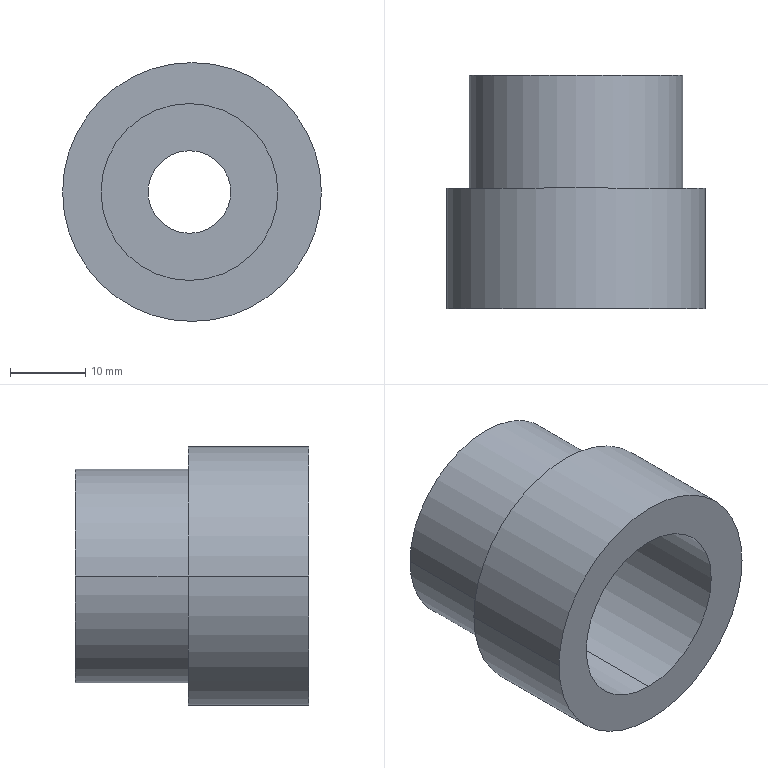Part | SolidWorks | features BaseBody 1, Scale 1 | 1 solid | 12 faces | box 34.39 x 31 x 34.39 mm | volume 12104 mm3 | cylinder 8 | plane 4 | commonest cylinder face diameters 11 x2 23.5 x2 28.4 x2 34.39 x2
STEP:
#1=CARTESIAN_POINT('',(0.,27.5,11.75));
#2=VERTEX_POINT('',#1);
#3=CARTESIAN_POINT('',(0.,27.5,-11.75));
#4=VERTEX_POINT('',#3);
#5=CARTESIAN_POINT('',(0.,27.5,0.));
#6=DIRECTION('',(0.,-1.,0.));
#7=DIRECTION('',(0.,0.,-1.));
#8=AXIS2_PLACEMENT_3D('',#5,#6,#7);
#9=CIRCLE('',#8,11.75);
#10=EDGE_CURVE('',#2,#4,#9,.T.);
#11=ORIENTED_EDGE('',*,*,#10,.F.);
#12=CARTESIAN_POINT('',(0.,0.,11.75));
#13=VERTEX_POINT('',#12);
#14=CARTESIAN_POINT('',(0.,27.5,11.75));
#15=DIRECTION('',(0.,-1.,0.));
#16=VECTOR('',#15,1000.);
#17=LINE('',#14,#16);
#18=EDGE_CURVE('',#2,#13,#17,.T.);
#19=ORIENTED_EDGE('',*,*,#18,.T.);
#20=CARTESIAN_POINT('',(0.,0.,-11.75));
#21=VERTEX_POINT('',#20);
#22=CARTESIAN_POINT('',(0.,0.,0.));
#23=DIRECTION('',(0.,1.,0.));
#24=DIRECTION('',(0.,0.,-1.));
#25=AXIS2_PLACEMENT_3D('',#22,#23,#24);
#26=CIRCLE('',#25,11.75);
#27=EDGE_CURVE('',#21,#13,#26,.T.);
#28=ORIENTED_EDGE('',*,*,#27,.F.);
#29=CARTESIAN_POINT('',(0.,27.5,-11.75));
#30=DIRECTION('',(0.,-1.,0.));
#31=VECTOR('',#30,1000.);
#32=LINE('',#29,#31);
#33=EDGE_CURVE('',#4,#21,#32,.T.);
#34=ORIENTED_EDGE('',*,*,#33,.F.);
#35=EDGE_LOOP('',(#11,#19,#28,#34));
#36=FACE_OUTER_BOUND('',#35,.T.);
#37=CARTESIAN_POINT('',(0.,27.5,0.));
#38=DIRECTION('',(0.,-1.,0.));
#39=DIRECTION('',(0.,0.,-1.));
#40=AXIS2_PLACEMENT_3D('',#37,#38,#39);
#41=CYLINDRICAL_SURFACE('',#40,11.75);
#42=ADVANCED_FACE('',(#36),#41,.F.);
#43=CARTESIAN_POINT('',(0.,27.5,-5.5));
#44=VERTEX_POINT('',#43);
#45=CARTESIAN_POINT('',(0.,27.5,5.5));
#46=VERTEX_POINT('',#45);
#47=CARTESIAN_POINT('',(0.,27.5,0.));
#48=DIRECTION('',(0.,1.,0.));
#49=DIRECTION('',(0.,0.,1.));
#50=AXIS2_PLACEMENT_3D('',#47,#48,#49);
#51=CIRCLE('',#50,5.5);
#52=EDGE_CURVE('',#44,#46,#51,.T.);
#53=ORIENTED_EDGE('',*,*,#52,.F.);
#54=CARTESIAN_POINT('',(0.,31.,-5.5));
#55=VERTEX_POINT('',#54);
#56=CARTESIAN_POINT('',(0.,7.5,-5.5));
#57=DIRECTION('',(0.,1.,0.));
#58=VECTOR('',#57,1000.);
#59=LINE('',#56,#58);
#60=EDGE_CURVE('',#44,#55,#59,.T.);
#61=ORIENTED_EDGE('',*,*,#60,.T.);
#62=CARTESIAN_POINT('',(0.,31.,5.5));
#63=VERTEX_POINT('',#62);
#64=CARTESIAN_POINT('',(0.,31.,0.));
#65=DIRECTION('',(0.,-1.,0.));
#66=DIRECTION('',(0.,0.,1.));
#67=AXIS2_PLACEMENT_3D('',#64,#65,#66);
#68=CIRCLE('',#67,5.5);
#69=EDGE_CURVE('',#63,#55,#68,.T.);
#70=ORIENTED_EDGE('',*,*,#69,.F.);
#71=CARTESIAN_POINT('',(0.,7.5,5.5));
#72=DIRECTION('',(0.,1.,0.));
#73=VECTOR('',#72,1000.);
#74=LINE('',#71,#73);
#75=EDGE_CURVE('',#46,#63,#74,.T.);
#76=ORIENTED_EDGE('',*,*,#75,.F.);
#77=EDGE_LOOP('',(#53,#61,#70,#76));
#78=FACE_OUTER_BOUND('',#77,.T.);
#79=CARTESIAN_POINT('',(0.,7.5,0.));
#80=DIRECTION('',(0.,1.,0.));
#81=DIRECTION('',(0.,0.,1.));
#82=AXIS2_PLACEMENT_3D('',#79,#80,#81);
#83=CYLINDRICAL_SURFACE('',#82,5.5);
#84=ADVANCED_FACE('',(#78),#83,.F.);
#85=CARTESIAN_POINT('',(17.533,0.,0.));
#86=VERTEX_POINT('',#85);
#87=CARTESIAN_POINT('',(-16.857,0.,0.));
#88=VERTEX_POINT('',#87);
#89=CARTESIAN_POINT('',(0.338,0.,0.));
#90=DIRECTION('',(0.,-1.,0.));
#91=DIRECTION('',(-1.,0.,0.));
#92=AXIS2_PLACEMENT_3D('',#89,#90,#91);
#93=CIRCLE('',#92,17.195);
#94=EDGE_CURVE('',#86,#88,#93,.T.);
#95=ORIENTED_EDGE('',*,*,#94,.F.);
#96=CARTESIAN_POINT('',(17.533,16.,0.));
#97=VERTEX_POINT('',#96);
#98=CARTESIAN_POINT('',(17.533,31.,0.));
#99=DIRECTION('',(0.,1.,0.));
#100=VECTOR('',#99,1000.);
#101=LINE('',#98,#100);
#102=EDGE_CURVE('',#86,#97,#101,.T.);
#103=ORIENTED_EDGE('',*,*,#102,.T.);
#104=CARTESIAN_POINT('',(-16.857,16.,0.));
#105=VERTEX_POINT('',#104);
#106=CARTESIAN_POINT('',(0.338,16.,0.));
#107=DIRECTION('',(0.,-1.,0.));
#108=DIRECTION('',(-1.,0.,0.));
#109=AXIS2_PLACEMENT_3D('',#106,#107,#108);
#110=CIRCLE('',#109,17.195);
#111=EDGE_CURVE('',#97,#105,#110,.T.);
#112=ORIENTED_EDGE('',*,*,#111,.T.);
#113=CARTESIAN_POINT('',(-16.857,31.,0.));
#114=DIRECTION('',(0.,1.,0.));
#115=VECTOR('',#114,1000.);
#116=LINE('',#113,#115);
#117=EDGE_CURVE('',#88,#105,#116,.T.);
#118=ORIENTED_EDGE('',*,*,#117,.F.);
#119=EDGE_LOOP('',(#95,#103,#112,#118));
#120=FACE_OUTER_BOUND('',#119,.T.);
#121=CARTESIAN_POINT('',(0.338,31.,0.));
#122=DIRECTION('',(0.,1.,0.));
#123=DIRECTION('',(-1.,0.,0.));
#124=AXIS2_PLACEMENT_3D('',#121,#122,#123);
#125=CYLINDRICAL_SURFACE('',#124,17.195);
#126=ADVANCED_FACE('',(#120),#125,.T.);
#127=CARTESIAN_POINT('',(14.538,16.,0.));
#128=VERTEX_POINT('',#127);
#129=CARTESIAN_POINT('',(-13.862,16.,0.));
#130=VERTEX_POINT('',#129);
#131=CARTESIAN_POINT('',(0.338,16.,0.));
#132=DIRECTION('',(0.,-1.,0.));
#133=DIRECTION('',(-1.,0.,0.));
#134=AXIS2_PLACEMENT_3D('',#131,#132,#133);
#135=CIRCLE('',#134,14.2);
#136=EDGE_CURVE('',#128,#130,#135,.T.);
#137=ORIENTED_EDGE('',*,*,#136,.F.);
#138=CARTESIAN_POINT('',(14.538,31.,0.));
#139=VERTEX_POINT('',#138);
#140=CARTESIAN_POINT('',(14.538,31.,0.));
#141=DIRECTION('',(0.,1.,0.));
#142=VECTOR('',#141,1000.);
#143=LINE('',#140,#142);
#144=EDGE_CURVE('',#128,#139,#143,.T.);
#145=ORIENTED_EDGE('',*,*,#144,.T.);
#146=CARTESIAN_POINT('',(-13.862,31.,0.));
#147=VERTEX_POINT('',#146);
#148=CARTESIAN_POINT('',(0.338,31.,0.));
#149=DIRECTION('',(0.,1.,0.));
#150=DIRECTION('',(-1.,0.,0.));
#151=AXIS2_PLACEMENT_3D('',#148,#149,#150);
#152=CIRCLE('',#151,14.2);
#153=EDGE_CURVE('',#147,#139,#152,.T.);
#154=ORIENTED_EDGE('',*,*,#153,.F.);
#155=CARTESIAN_POINT('',(-13.862,31.,0.));
#156=DIRECTION('',(0.,1.,0.));
#157=VECTOR('',#156,1000.);
#158=LINE('',#155,#157);
#159=EDGE_CURVE('',#130,#147,#158,.T.);
#160=ORIENTED_EDGE('',*,*,#159,.F.);
#161=EDGE_LOOP('',(#137,#145,#154,#160));
#162=FACE_OUTER_BOUND('',#161,.T.);
#163=CARTESIAN_POINT('',(0.338,31.,0.));
#164=DIRECTION('',(0.,1.,0.));
#165=DIRECTION('',(-1.,0.,0.));
#166=AXIS2_PLACEMENT_3D('',#163,#164,#165);
#167=CYLINDRICAL_SURFACE('',#166,14.2);
#168=ADVANCED_FACE('',(#162),#167,.T.);
#169=ORIENTED_EDGE('',*,*,#18,.F.);
#170=CARTESIAN_POINT('',(0.,27.5,0.));
#171=DIRECTION('',(0.,-1.,0.));
#172=DIRECTION('',(0.,0.,-1.));
#173=AXIS2_PLACEMENT_3D('',#170,#171,#172);
#174=CIRCLE('',#173,11.75);
#175=EDGE_CURVE('',#4,#2,#174,.T.);
#176=ORIENTED_EDGE('',*,*,#175,.F.);
#177=ORIENTED_EDGE('',*,*,#33,.T.);
#178=CARTESIAN_POINT('',(0.,0.,0.));
#179=DIRECTION('',(0.,1.,0.));
#180=DIRECTION('',(0.,0.,-1.));
#181=AXIS2_PLACEMENT_3D('',#178,#179,#180);
#182=CIRCLE('',#181,11.75);
#183=EDGE_CURVE('',#13,#21,#182,.T.);
#184=ORIENTED_EDGE('',*,*,#183,.F.);
#185=EDGE_LOOP('',(#169,#176,#177,#184));
#186=FACE_OUTER_BOUND('',#185,.T.);
#187=CARTESIAN_POINT('',(0.,27.5,0.));
#188=DIRECTION('',(0.,-1.,0.));
#189=DIRECTION('',(0.,0.,-1.));
#190=AXIS2_PLACEMENT_3D('',#187,#188,#189);
#191=CYLINDRICAL_SURFACE('',#190,11.75);
#192=ADVANCED_FACE('',(#186),#191,.F.);
#193=CARTESIAN_POINT('',(0.,27.5,0.));
#194=DIRECTION('',(0.,1.,0.));
#195=DIRECTION('',(0.,0.,1.));
#196=AXIS2_PLACEMENT_3D('',#193,#194,#195);
#197=CIRCLE('',#196,5.5);
#198=EDGE_CURVE('',#46,#44,#197,.T.);
#199=ORIENTED_EDGE('',*,*,#198,.T.);
#200=ORIENTED_EDGE('',*,*,#52,.T.);
#201=EDGE_LOOP('',(#199,#200));
#202=FACE_BOUND('',#201,.T.);
#203=ORIENTED_EDGE('',*,*,#175,.T.);
#204=ORIENTED_EDGE('',*,*,#10,.T.);
#205=EDGE_LOOP('',(#203,#204));
#206=FACE_OUTER_BOUND('',#205,.T.);
#207=CARTESIAN_POINT('',(0.,27.5,0.));
#208=DIRECTION('',(0.,-1.,0.));
#209=DIRECTION('',(0.,0.,-1.));
#210=AXIS2_PLACEMENT_3D('',#207,#208,#209);
#211=PLANE('',#210);
#212=ADVANCED_FACE('',(#202,#206),#211,.T.);
#213=ORIENTED_EDGE('',*,*,#27,.T.);
#214=ORIENTED_EDGE('',*,*,#183,.T.);
#215=EDGE_LOOP('',(#213,#214));
#216=FACE_BOUND('',#215,.T.);
#217=CARTESIAN_POINT('',(0.338,0.,0.));
#218=DIRECTION('',(0.,-1.,0.));
#219=DIRECTION('',(-1.,0.,0.));
#220=AXIS2_PLACEMENT_3D('',#217,#218,#219);
#221=CIRCLE('',#220,17.195);
#222=EDGE_CURVE('',#88,#86,#221,.T.);
#223=ORIENTED_EDGE('',*,*,#222,.T.);
#224=ORIENTED_EDGE('',*,*,#94,.T.);
#225=EDGE_LOOP('',(#223,#224));
#226=FACE_OUTER_BOUND('',#225,.T.);
#227=CARTESIAN_POINT('',(0.338,0.,0.));
#228=DIRECTION('',(0.,-1.,0.));
#229=DIRECTION('',(1.,0.,0.));
#230=AXIS2_PLACEMENT_3D('',#227,#228,#229);
#231=PLANE('',#230);
#232=ADVANCED_FACE('',(#216,#226),#231,.T.);
#233=ORIENTED_EDGE('',*,*,#60,.F.);
#234=ORIENTED_EDGE('',*,*,#198,.F.);
#235=ORIENTED_EDGE('',*,*,#75,.T.);
#236=CARTESIAN_POINT('',(0.,31.,0.));
#237=DIRECTION('',(0.,-1.,0.));
#238=DIRECTION('',(0.,0.,1.));
#239=AXIS2_PLACEMENT_3D('',#236,#237,#238);
#240=CIRCLE('',#239,5.5);
#241=EDGE_CURVE('',#55,#63,#240,.T.);
#242=ORIENTED_EDGE('',*,*,#241,.F.);
#243=EDGE_LOOP('',(#233,#234,#235,#242));
#244=FACE_OUTER_BOUND('',#243,.T.);
#245=CARTESIAN_POINT('',(0.,7.5,0.));
#246=DIRECTION('',(0.,1.,0.));
#247=DIRECTION('',(0.,0.,1.));
#248=AXIS2_PLACEMENT_3D('',#245,#246,#247);
#249=CYLINDRICAL_SURFACE('',#248,5.5);
#250=ADVANCED_FACE('',(#244),#249,.F.);
#251=ORIENTED_EDGE('',*,*,#102,.F.);
#252=ORIENTED_EDGE('',*,*,#222,.F.);
#253=ORIENTED_EDGE('',*,*,#117,.T.);
#254=CARTESIAN_POINT('',(0.338,16.,0.));
#255=DIRECTION('',(0.,-1.,0.));
#256=DIRECTION('',(-1.,0.,0.));
#257=AXIS2_PLACEMENT_3D('',#254,#255,#256);
#258=CIRCLE('',#257,17.195);
#259=EDGE_CURVE('',#105,#97,#258,.T.);
#260=ORIENTED_EDGE('',*,*,#259,.T.);
#261=EDGE_LOOP('',(#251,#252,#253,#260));
#262=FACE_OUTER_BOUND('',#261,.T.);
#263=CARTESIAN_POINT('',(0.338,31.,0.));
#264=DIRECTION('',(0.,1.,0.));
#265=DIRECTION('',(-1.,0.,0.));
#266=AXIS2_PLACEMENT_3D('',#263,#264,#265);
#267=CYLINDRICAL_SURFACE('',#266,17.195);
#268=ADVANCED_FACE('',(#262),#267,.T.);
#269=ORIENTED_EDGE('',*,*,#69,.T.);
#270=ORIENTED_EDGE('',*,*,#241,.T.);
#271=EDGE_LOOP('',(#269,#270));
#272=FACE_BOUND('',#271,.T.);
#273=ORIENTED_EDGE('',*,*,#153,.T.);
#274=CARTESIAN_POINT('',(0.338,31.,0.));
#275=DIRECTION('',(0.,1.,0.));
#276=DIRECTION('',(-1.,0.,0.));
#277=AXIS2_PLACEMENT_3D('',#274,#275,#276);
#278=CIRCLE('',#277,14.2);
#279=EDGE_CURVE('',#139,#147,#278,.T.);
#280=ORIENTED_EDGE('',*,*,#279,.T.);
#281=EDGE_LOOP('',(#273,#280));
#282=FACE_OUTER_BOUND('',#281,.T.);
#283=CARTESIAN_POINT('',(0.338,31.,0.));
#284=DIRECTION('',(0.,1.,0.));
#285=DIRECTION('',(-1.,0.,0.));
#286=AXIS2_PLACEMENT_3D('',#283,#284,#285);
#287=PLANE('',#286);
#288=ADVANCED_FACE('',(#272,#282),#287,.T.);
#289=CARTESIAN_POINT('',(0.338,16.,0.));
#290=DIRECTION('',(0.,-1.,0.));
#291=DIRECTION('',(-1.,0.,0.));
#292=AXIS2_PLACEMENT_3D('',#289,#290,#291);
#293=CIRCLE('',#292,14.2);
#294=EDGE_CURVE('',#130,#128,#293,.T.);
#295=ORIENTED_EDGE('',*,*,#294,.T.);
#296=ORIENTED_EDGE('',*,*,#136,.T.);
#297=EDGE_LOOP('',(#295,#296));
#298=FACE_BOUND('',#297,.T.);
#299=ORIENTED_EDGE('',*,*,#259,.F.);
#300=ORIENTED_EDGE('',*,*,#111,.F.);
#301=EDGE_LOOP('',(#299,#300));
#302=FACE_OUTER_BOUND('',#301,.T.);
#303=CARTESIAN_POINT('',(14.538,16.,0.));
#304=DIRECTION('',(0.,1.,0.));
#305=DIRECTION('',(-1.,0.,0.));
#306=AXIS2_PLACEMENT_3D('',#303,#304,#305);
#307=PLANE('',#306);
#308=ADVANCED_FACE('',(#298,#302),#307,.T.);
#309=ORIENTED_EDGE('',*,*,#144,.F.);
#310=ORIENTED_EDGE('',*,*,#294,.F.);
#311=ORIENTED_EDGE('',*,*,#159,.T.);
#312=ORIENTED_EDGE('',*,*,#279,.F.);
#313=EDGE_LOOP('',(#309,#310,#311,#312));
#314=FACE_OUTER_BOUND('',#313,.T.);
#315=CARTESIAN_POINT('',(0.338,31.,0.));
#316=DIRECTION('',(0.,1.,0.));
#317=DIRECTION('',(-1.,0.,0.));
#318=AXIS2_PLACEMENT_3D('',#315,#316,#317);
#319=CYLINDRICAL_SURFACE('',#318,14.2);
#320=ADVANCED_FACE('',(#314),#319,.T.);
#321=CLOSED_SHELL('',(#42,#84,#126,#168,#192,#212,#232,#250,#268,#288,#308,#320));
#322=MANIFOLD_SOLID_BREP('',#321);
#323=CARTESIAN_POINT('',(0.,0.,0.));
#324=DIRECTION('',(0.,0.,1.));
#325=DIRECTION('',(1.,0.,0.));
#326=AXIS2_PLACEMENT_3D('',#323,#324,#325);
#327=(LENGTH_UNIT()NAMED_UNIT(*)SI_UNIT(.MILLI.,.METRE.));
#328=UNCERTAINTY_MEASURE_WITH_UNIT(LENGTH_MEASURE(0.00001),#327,'','');
#329=(NAMED_UNIT(*)PLANE_ANGLE_UNIT()SI_UNIT($,.RADIAN.));
#330=(NAMED_UNIT(*)SI_UNIT($,.STERADIAN.)SOLID_ANGLE_UNIT());
#331=(GEOMETRIC_REPRESENTATION_CONTEXT(3)GLOBAL_UNCERTAINTY_ASSIGNED_CONTEXT((#328))GLOBAL_UNIT_ASSIGNED_CONTEXT((#327,#329,#330))REPRESENTATION_CONTEXT('',''));
#332=ADVANCED_BREP_SHAPE_REPRESENTATION('',(#322,#326),#331);